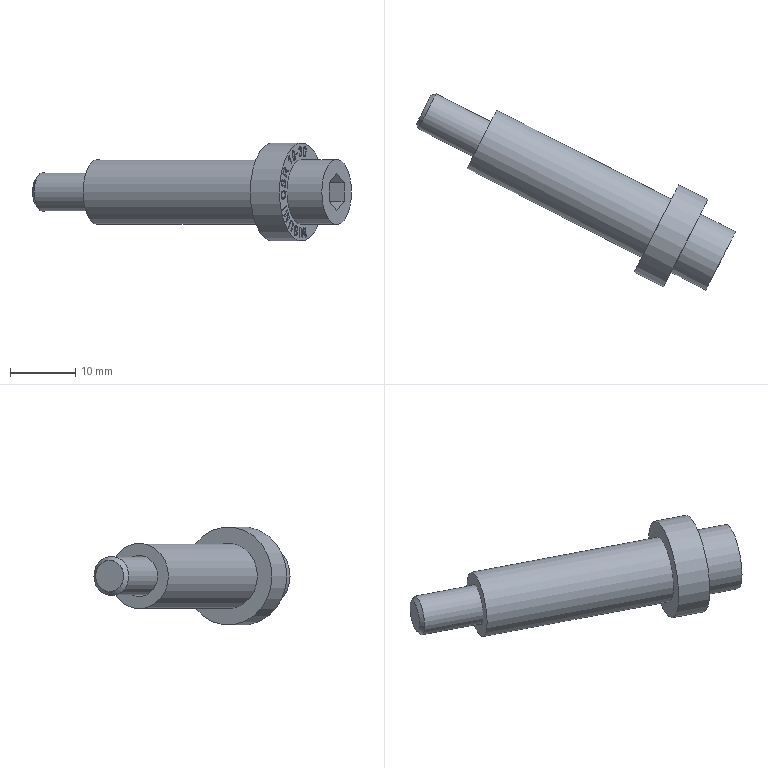Part | STEP file | gslz 2016.10.28-13_id1794_x_t | 1 solid | 208 faces | box 48.801 x 30.009 x 15 mm | volume 3814 mm3 | other 109 | plane 91 | cylinder 7 | cone 1 | commonest cylinder face diameters 10 x2 4.8 x1 4.82 x1 6 x1 6.3 x1 15 x1